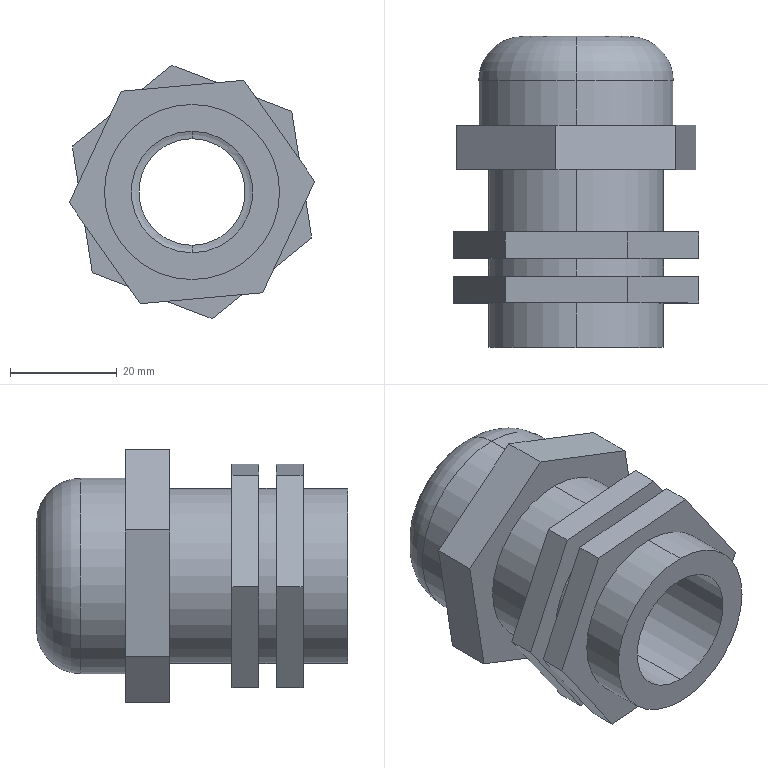Part | SolidWorks | features ICE 5, Extrusion 1, Fillet 1, Scale 1, Shell 1 | 1 solid | 44 faces | box 46.006 x 58.333 x 47.523 mm | volume 36742 mm3 | plane 26 | cylinder 14 | torus 4 | commonest cylinder face diameters 32.833 x6 20 x2 22.833 x2 26.667 x2 36.667 x2
STEP:
#1=CARTESIAN_POINT('',(0.,26.887,-11.417));
#2=VERTEX_POINT('',#1);
#3=CARTESIAN_POINT('',(0.,26.887,11.417));
#4=VERTEX_POINT('',#3);
#5=CARTESIAN_POINT('',(0.,26.887,0.));
#6=DIRECTION('',(0.,1.,0.));
#7=DIRECTION('',(0.,0.,1.));
#8=AXIS2_PLACEMENT_3D('',#5,#6,#7);
#9=CIRCLE('',#8,11.417);
#10=EDGE_CURVE('',#2,#4,#9,.T.);
#11=ORIENTED_EDGE('',*,*,#10,.T.);
#12=CARTESIAN_POINT('',(0.,-11.447,11.417));
#13=VERTEX_POINT('',#12);
#14=CARTESIAN_POINT('',(0.,21.887,11.417));
#15=DIRECTION('',(0.,-1.,0.));
#16=VECTOR('',#15,1000.);
#17=LINE('',#14,#16);
#18=EDGE_CURVE('',#4,#13,#17,.T.);
#19=ORIENTED_EDGE('',*,*,#18,.T.);
#20=CARTESIAN_POINT('',(0.,-11.447,-11.417));
#21=VERTEX_POINT('',#20);
#22=CARTESIAN_POINT('',(0.,-11.447,0.));
#23=DIRECTION('',(0.,1.,0.));
#24=DIRECTION('',(0.,0.,1.));
#25=AXIS2_PLACEMENT_3D('',#22,#23,#24);
#26=CIRCLE('',#25,11.417);
#27=EDGE_CURVE('',#21,#13,#26,.T.);
#28=ORIENTED_EDGE('',*,*,#27,.F.);
#29=CARTESIAN_POINT('',(0.,21.887,-11.417));
#30=DIRECTION('',(0.,-1.,0.));
#31=VECTOR('',#30,1000.);
#32=LINE('',#29,#31);
#33=EDGE_CURVE('',#2,#21,#32,.T.);
#34=ORIENTED_EDGE('',*,*,#33,.F.);
#35=EDGE_LOOP('',(#11,#19,#28,#34));
#36=FACE_OUTER_BOUND('',#35,.T.);
#37=CARTESIAN_POINT('',(0.,21.887,0.));
#38=DIRECTION('',(0.,-1.,0.));
#39=DIRECTION('',(0.,0.,-1.));
#40=AXIS2_PLACEMENT_3D('',#37,#38,#39);
#41=CYLINDRICAL_SURFACE('',#40,11.417);
#42=ADVANCED_FACE('',(#36),#41,.F.);
#43=CARTESIAN_POINT('',(0.,-3.113,-16.417));
#44=VERTEX_POINT('',#43);
#45=CARTESIAN_POINT('',(0.,-3.113,16.417));
#46=VERTEX_POINT('',#45);
#47=CARTESIAN_POINT('',(0.,-3.113,0.));
#48=DIRECTION('',(0.,-1.,0.));
#49=DIRECTION('',(0.,0.,-1.));
#50=AXIS2_PLACEMENT_3D('',#47,#48,#49);
#51=CIRCLE('',#50,16.417);
#52=EDGE_CURVE('',#44,#46,#51,.T.);
#53=ORIENTED_EDGE('',*,*,#52,.T.);
#54=CARTESIAN_POINT('',(0.,-11.447,16.417));
#55=VERTEX_POINT('',#54);
#56=CARTESIAN_POINT('',(0.,21.887,16.417));
#57=DIRECTION('',(0.,-1.,0.));
#58=VECTOR('',#57,1000.);
#59=LINE('',#56,#58);
#60=EDGE_CURVE('',#46,#55,#59,.T.);
#61=ORIENTED_EDGE('',*,*,#60,.T.);
#62=CARTESIAN_POINT('',(0.,-11.447,-16.417));
#63=VERTEX_POINT('',#62);
#64=CARTESIAN_POINT('',(0.,-11.447,0.));
#65=DIRECTION('',(0.,1.,0.));
#66=DIRECTION('',(0.,0.,1.));
#67=AXIS2_PLACEMENT_3D('',#64,#65,#66);
#68=CIRCLE('',#67,16.417);
#69=EDGE_CURVE('',#55,#63,#68,.T.);
#70=ORIENTED_EDGE('',*,*,#69,.T.);
#71=CARTESIAN_POINT('',(0.,21.887,-16.417));
#72=DIRECTION('',(0.,-1.,0.));
#73=VECTOR('',#72,1000.);
#74=LINE('',#71,#73);
#75=EDGE_CURVE('',#44,#63,#74,.T.);
#76=ORIENTED_EDGE('',*,*,#75,.F.);
#77=EDGE_LOOP('',(#53,#61,#70,#76));
#78=FACE_OUTER_BOUND('',#77,.T.);
#79=CARTESIAN_POINT('',(0.,21.887,0.));
#80=DIRECTION('',(0.,-1.,0.));
#81=DIRECTION('',(0.,0.,-1.));
#82=AXIS2_PLACEMENT_3D('',#79,#80,#81);
#83=CYLINDRICAL_SURFACE('',#82,16.417);
#84=ADVANCED_FACE('',(#78),#83,.T.);
#85=CARTESIAN_POINT('',(0.,38.553,13.333));
#86=VERTEX_POINT('',#85);
#87=CARTESIAN_POINT('',(0.,38.553,-13.333));
#88=VERTEX_POINT('',#87);
#89=CARTESIAN_POINT('',(0.,38.553,0.));
#90=DIRECTION('',(0.,-1.,0.));
#91=DIRECTION('',(0.,0.,-1.));
#92=AXIS2_PLACEMENT_3D('',#89,#90,#91);
#93=CIRCLE('',#92,13.333);
#94=EDGE_CURVE('',#86,#88,#93,.T.);
#95=ORIENTED_EDGE('',*,*,#94,.T.);
#96=CARTESIAN_POINT('',(0.,41.887,-10.));
#97=VERTEX_POINT('',#96);
#98=CARTESIAN_POINT('',(0.,38.553,-10.));
#99=DIRECTION('',(1.,0.,0.));
#100=DIRECTION('',(0.,0.,-1.));
#101=AXIS2_PLACEMENT_3D('',#98,#99,#100);
#102=CIRCLE('',#101,3.333);
#103=EDGE_CURVE('',#88,#97,#102,.T.);
#104=ORIENTED_EDGE('',*,*,#103,.T.);
#105=CARTESIAN_POINT('',(0.,41.887,10.));
#106=VERTEX_POINT('',#105);
#107=CARTESIAN_POINT('',(0.,41.887,0.));
#108=DIRECTION('',(0.,1.,0.));
#109=DIRECTION('',(0.,0.,-1.));
#110=AXIS2_PLACEMENT_3D('',#107,#108,#109);
#111=CIRCLE('',#110,10.);
#112=EDGE_CURVE('',#97,#106,#111,.T.);
#113=ORIENTED_EDGE('',*,*,#112,.T.);
#114=CARTESIAN_POINT('',(0.,38.553,10.));
#115=DIRECTION('',(-1.,0.,0.));
#116=DIRECTION('',(0.,0.,1.));
#117=AXIS2_PLACEMENT_3D('',#114,#115,#116);
#118=CIRCLE('',#117,3.333);
#119=EDGE_CURVE('',#86,#106,#118,.T.);
#120=ORIENTED_EDGE('',*,*,#119,.F.);
#121=EDGE_LOOP('',(#95,#104,#113,#120));
#122=FACE_OUTER_BOUND('',#121,.T.);
#123=CARTESIAN_POINT('',(0.,38.553,0.));
#124=DIRECTION('',(0.,1.,0.));
#125=DIRECTION('',(0.,0.,1.));
#126=AXIS2_PLACEMENT_3D('',#123,#124,#125);
#127=TOROIDAL_SURFACE('',#126,10.,3.333);
#128=ADVANCED_FACE('',(#122),#127,.F.);
#129=ORIENTED_EDGE('',*,*,#94,.F.);
#130=CARTESIAN_POINT('',(0.,26.887,13.333));
#131=VERTEX_POINT('',#130);
#132=CARTESIAN_POINT('',(0.,46.887,13.333));
#133=DIRECTION('',(0.,-1.,0.));
#134=VECTOR('',#133,1000.);
#135=LINE('',#132,#134);
#136=EDGE_CURVE('',#86,#131,#135,.T.);
#137=ORIENTED_EDGE('',*,*,#136,.T.);
#138=CARTESIAN_POINT('',(0.,26.887,-13.333));
#139=VERTEX_POINT('',#138);
#140=CARTESIAN_POINT('',(0.,26.887,0.));
#141=DIRECTION('',(0.,-1.,0.));
#142=DIRECTION('',(0.,0.,1.));
#143=AXIS2_PLACEMENT_3D('',#140,#141,#142);
#144=CIRCLE('',#143,13.333);
#145=EDGE_CURVE('',#131,#139,#144,.T.);
#146=ORIENTED_EDGE('',*,*,#145,.T.);
#147=CARTESIAN_POINT('',(0.,46.887,-13.333));
#148=DIRECTION('',(0.,-1.,0.));
#149=VECTOR('',#148,1000.);
#150=LINE('',#147,#149);
#151=EDGE_CURVE('',#88,#139,#150,.T.);
#152=ORIENTED_EDGE('',*,*,#151,.F.);
#153=EDGE_LOOP('',(#129,#137,#146,#152));
#154=FACE_OUTER_BOUND('',#153,.T.);
#155=CARTESIAN_POINT('',(0.,46.887,0.));
#156=DIRECTION('',(0.,-1.,0.));
#157=DIRECTION('',(0.,0.,-1.));
#158=AXIS2_PLACEMENT_3D('',#155,#156,#157);
#159=CYLINDRICAL_SURFACE('',#158,13.333);
#160=ADVANCED_FACE('',(#154),#159,.F.);
#161=ORIENTED_EDGE('',*,*,#112,.F.);
#162=CARTESIAN_POINT('',(0.,46.887,-10.));
#163=VERTEX_POINT('',#162);
#164=CARTESIAN_POINT('',(0.,46.887,-10.));
#165=DIRECTION('',(0.,1.,0.));
#166=VECTOR('',#165,1000.);
#167=LINE('',#164,#166);
#168=EDGE_CURVE('',#97,#163,#167,.T.);
#169=ORIENTED_EDGE('',*,*,#168,.T.);
#170=CARTESIAN_POINT('',(0.,46.887,10.));
#171=VERTEX_POINT('',#170);
#172=CARTESIAN_POINT('',(0.,46.887,0.));
#173=DIRECTION('',(0.,1.,0.));
#174=DIRECTION('',(0.,0.,1.));
#175=AXIS2_PLACEMENT_3D('',#172,#173,#174);
#176=CIRCLE('',#175,10.);
#177=EDGE_CURVE('',#163,#171,#176,.T.);
#178=ORIENTED_EDGE('',*,*,#177,.T.);
#179=CARTESIAN_POINT('',(0.,46.887,10.));
#180=DIRECTION('',(0.,1.,0.));
#181=VECTOR('',#180,1000.);
#182=LINE('',#179,#181);
#183=EDGE_CURVE('',#106,#171,#182,.T.);
#184=ORIENTED_EDGE('',*,*,#183,.F.);
#185=EDGE_LOOP('',(#161,#169,#178,#184));
#186=FACE_OUTER_BOUND('',#185,.T.);
#187=CARTESIAN_POINT('',(0.,46.887,0.));
#188=DIRECTION('',(0.,1.,0.));
#189=DIRECTION('',(0.,0.,1.));
#190=AXIS2_PLACEMENT_3D('',#187,#188,#189);
#191=CYLINDRICAL_SURFACE('',#190,10.);
#192=ADVANCED_FACE('',(#186),#191,.F.);
#193=CARTESIAN_POINT('',(0.,38.553,-18.333));
#194=VERTEX_POINT('',#193);
#195=CARTESIAN_POINT('',(0.,38.553,18.333));
#196=VERTEX_POINT('',#195);
#197=CARTESIAN_POINT('',(0.,38.553,0.));
#198=DIRECTION('',(0.,-1.,0.));
#199=DIRECTION('',(0.,0.,1.));
#200=AXIS2_PLACEMENT_3D('',#197,#198,#199);
#201=CIRCLE('',#200,18.333);
#202=EDGE_CURVE('',#194,#196,#201,.T.);
#203=ORIENTED_EDGE('',*,*,#202,.F.);
#204=CARTESIAN_POINT('',(0.,38.553,-10.));
#205=DIRECTION('',(1.,0.,0.));
#206=DIRECTION('',(0.,0.,-1.));
#207=AXIS2_PLACEMENT_3D('',#204,#205,#206);
#208=CIRCLE('',#207,8.333);
#209=EDGE_CURVE('',#194,#163,#208,.T.);
#210=ORIENTED_EDGE('',*,*,#209,.T.);
#211=CARTESIAN_POINT('',(0.,46.887,0.));
#212=DIRECTION('',(0.,1.,0.));
#213=DIRECTION('',(0.,0.,1.));
#214=AXIS2_PLACEMENT_3D('',#211,#212,#213);
#215=CIRCLE('',#214,10.);
#216=EDGE_CURVE('',#171,#163,#215,.T.);
#217=ORIENTED_EDGE('',*,*,#216,.F.);
#218=CARTESIAN_POINT('',(0.,38.553,10.));
#219=DIRECTION('',(-1.,0.,0.));
#220=DIRECTION('',(0.,0.,1.));
#221=AXIS2_PLACEMENT_3D('',#218,#219,#220);
#222=CIRCLE('',#221,8.333);
#223=EDGE_CURVE('',#196,#171,#222,.T.);
#224=ORIENTED_EDGE('',*,*,#223,.F.);
#225=EDGE_LOOP('',(#203,#210,#217,#224));
#226=FACE_OUTER_BOUND('',#225,.T.);
#227=CARTESIAN_POINT('',(0.,38.553,0.));
#228=DIRECTION('',(0.,1.,0.));
#229=DIRECTION('',(0.,0.,1.));
#230=AXIS2_PLACEMENT_3D('',#227,#228,#229);
#231=TOROIDAL_SURFACE('',#230,10.,8.333);
#232=ADVANCED_FACE('',(#226),#231,.T.);
#233=ORIENTED_EDGE('',*,*,#202,.T.);
#234=CARTESIAN_POINT('',(0.,30.22,18.333));
#235=VERTEX_POINT('',#234);
#236=CARTESIAN_POINT('',(0.,46.887,18.333));
#237=DIRECTION('',(0.,-1.,0.));
#238=VECTOR('',#237,1000.);
#239=LINE('',#236,#238);
#240=EDGE_CURVE('',#196,#235,#239,.T.);
#241=ORIENTED_EDGE('',*,*,#240,.T.);
#242=CARTESIAN_POINT('',(0.,30.22,-18.333));
#243=VERTEX_POINT('',#242);
#244=CARTESIAN_POINT('',(0.,30.22,0.));
#245=DIRECTION('',(0.,1.,0.));
#246=DIRECTION('',(0.,0.,1.));
#247=AXIS2_PLACEMENT_3D('',#244,#245,#246);
#248=CIRCLE('',#247,18.333);
#249=EDGE_CURVE('',#235,#243,#248,.T.);
#250=ORIENTED_EDGE('',*,*,#249,.T.);
#251=CARTESIAN_POINT('',(0.,46.887,-18.333));
#252=DIRECTION('',(0.,-1.,0.));
#253=VECTOR('',#252,1000.);
#254=LINE('',#251,#253);
#255=EDGE_CURVE('',#194,#243,#254,.T.);
#256=ORIENTED_EDGE('',*,*,#255,.F.);
#257=EDGE_LOOP('',(#233,#241,#250,#256));
#258=FACE_OUTER_BOUND('',#257,.T.);
#259=CARTESIAN_POINT('',(0.,46.887,0.));
#260=DIRECTION('',(0.,-1.,0.));
#261=DIRECTION('',(0.,0.,-1.));
#262=AXIS2_PLACEMENT_3D('',#259,#260,#261);
#263=CYLINDRICAL_SURFACE('',#262,18.333);
#264=ADVANCED_FACE('',(#258),#263,.T.);
#265=CARTESIAN_POINT('',(0.,21.887,16.417));
#266=VERTEX_POINT('',#265);
#267=CARTESIAN_POINT('',(0.,21.887,-16.417));
#268=VERTEX_POINT('',#267);
#269=CARTESIAN_POINT('',(0.,21.887,0.));
#270=DIRECTION('',(0.,1.,0.));
#271=DIRECTION('',(0.,0.,1.));
#272=AXIS2_PLACEMENT_3D('',#269,#270,#271);
#273=CIRCLE('',#272,16.417);
#274=EDGE_CURVE('',#266,#268,#273,.T.);
#275=ORIENTED_EDGE('',*,*,#274,.F.);
#276=CARTESIAN_POINT('',(0.,10.22,16.417));
#277=VERTEX_POINT('',#276);
#278=CARTESIAN_POINT('',(0.,21.887,16.417));
#279=DIRECTION('',(0.,-1.,0.));
#280=VECTOR('',#279,1000.);
#281=LINE('',#278,#280);
#282=EDGE_CURVE('',#266,#277,#281,.T.);
#283=ORIENTED_EDGE('',*,*,#282,.T.);
#284=CARTESIAN_POINT('',(0.,10.22,-16.417));
#285=VERTEX_POINT('',#284);
#286=CARTESIAN_POINT('',(0.,10.22,0.));
#287=DIRECTION('',(0.,-1.,0.));
#288=DIRECTION('',(0.,0.,-1.));
#289=AXIS2_PLACEMENT_3D('',#286,#287,#288);
#290=CIRCLE('',#289,16.417);
#291=EDGE_CURVE('',#285,#277,#290,.T.);
#292=ORIENTED_EDGE('',*,*,#291,.F.);
#293=CARTESIAN_POINT('',(0.,21.887,-16.417));
#294=DIRECTION('',(0.,-1.,0.));
#295=VECTOR('',#294,1000.);
#296=LINE('',#293,#295);
#297=EDGE_CURVE('',#268,#285,#296,.T.);
#298=ORIENTED_EDGE('',*,*,#297,.F.);
#299=EDGE_LOOP('',(#275,#283,#292,#298));
#300=FACE_OUTER_BOUND('',#299,.T.);
#301=CARTESIAN_POINT('',(0.,21.887,0.));
#302=DIRECTION('',(0.,-1.,0.));
#303=DIRECTION('',(0.,0.,-1.));
#304=AXIS2_PLACEMENT_3D('',#301,#302,#303);
#305=CYLINDRICAL_SURFACE('',#304,16.417);
#306=ADVANCED_FACE('',(#300),#305,.T.);
#307=CARTESIAN_POINT('',(0.,5.22,-16.417));
#308=VERTEX_POINT('',#307);
#309=CARTESIAN_POINT('',(0.,5.22,16.417));
#310=VERTEX_POINT('',#309);
#311=CARTESIAN_POINT('',(0.,5.22,0.));
#312=DIRECTION('',(0.,-1.,0.));
#313=DIRECTION('',(0.,0.,-1.));
#314=AXIS2_PLACEMENT_3D('',#311,#312,#313);
#315=CIRCLE('',#314,16.417);
#316=EDGE_CURVE('',#308,#310,#315,.T.);
#317=ORIENTED_EDGE('',*,*,#316,.T.);
#318=CARTESIAN_POINT('',(0.,1.887,16.417));
#319=VERTEX_POINT('',#318);
#320=CARTESIAN_POINT('',(0.,21.887,16.417));
#321=DIRECTION('',(0.,-1.,0.));
#322=VECTOR('',#321,1000.);
#323=LINE('',#320,#322);
#324=EDGE_CURVE('',#310,#319,#323,.T.);
#325=ORIENTED_EDGE('',*,*,#324,.T.);
#326=CARTESIAN_POINT('',(0.,1.887,-16.417));
#327=VERTEX_POINT('',#326);
#328=CARTESIAN_POINT('',(0.,1.887,0.));
#329=DIRECTION('',(0.,-1.,0.));
#330=DIRECTION('',(0.,0.,-1.));
#331=AXIS2_PLACEMENT_3D('',#328,#329,#330);
#332=CIRCLE('',#331,16.417);
#333=EDGE_CURVE('',#327,#319,#332,.T.);
#334=ORIENTED_EDGE('',*,*,#333,.F.);
#335=CARTESIAN_POINT('',(0.,21.887,-16.417));
#336=DIRECTION('',(0.,-1.,0.));
#337=VECTOR('',#336,1000.);
#338=LINE('',#335,#337);
#339=EDGE_CURVE('',#308,#327,#338,.T.);
#340=ORIENTED_EDGE('',*,*,#339,.F.);
#341=EDGE_LOOP('',(#317,#325,#334,#340));
#342=FACE_OUTER_BOUND('',#341,.T.);
#343=CARTESIAN_POINT('',(0.,21.887,0.));
#344=DIRECTION('',(0.,-1.,0.));
#345=DIRECTION('',(0.,0.,-1.));
#346=AXIS2_PLACEMENT_3D('',#343,#344,#345);
#347=CYLINDRICAL_SURFACE('',#346,16.417);
#348=ADVANCED_FACE('',(#342),#347,.T.);
#349=ORIENTED_EDGE('',*,*,#324,.F.);
#350=CARTESIAN_POINT('',(0.,5.22,0.));
#351=DIRECTION('',(0.,-1.,0.));
#352=DIRECTION('',(0.,0.,-1.));
#353=AXIS2_PLACEMENT_3D('',#350,#351,#352);
#354=CIRCLE('',#353,16.417);
#355=EDGE_CURVE('',#310,#308,#354,.T.);
#356=ORIENTED_EDGE('',*,*,#355,.T.);
#357=ORIENTED_EDGE('',*,*,#339,.T.);
#358=CARTESIAN_POINT('',(0.,1.887,0.));
#359=DIRECTION('',(0.,-1.,0.));
#360=DIRECTION('',(0.,0.,-1.));
#361=AXIS2_PLACEMENT_3D('',#358,#359,#360);
#362=CIRCLE('',#361,16.417);
#363=EDGE_CURVE('',#319,#327,#362,.T.);
#364=ORIENTED_EDGE('',*,*,#363,.F.);
#365=EDGE_LOOP('',(#349,#356,#357,#364));
#366=FACE_OUTER_BOUND('',#365,.T.);
#367=CARTESIAN_POINT('',(0.,21.887,0.));
#368=DIRECTION('',(0.,-1.,0.));
#369=DIRECTION('',(0.,0.,-1.));
#370=AXIS2_PLACEMENT_3D('',#367,#368,#369);
#371=CYLINDRICAL_SURFACE('',#370,16.417);
#372=ADVANCED_FACE('',(#366),#371,.T.);
#373=ORIENTED_EDGE('',*,*,#282,.F.);
#374=CARTESIAN_POINT('',(0.,21.887,0.));
#375=DIRECTION('',(0.,1.,0.));
#376=DIRECTION('',(0.,0.,1.));
#377=AXIS2_PLACEMENT_3D('',#374,#375,#376);
#378=CIRCLE('',#377,16.417);
#379=EDGE_CURVE('',#268,#266,#378,.T.);
#380=ORIENTED_EDGE('',*,*,#379,.F.);
#381=ORIENTED_EDGE('',*,*,#297,.T.);
#382=CARTESIAN_POINT('',(0.,10.22,0.));
#383=DIRECTION('',(0.,-1.,0.));
#384=DIRECTION('',(0.,0.,-1.));
#385=AXIS2_PLACEMENT_3D('',#382,#383,#384);
#386=CIRCLE('',#385,16.417);
#387=EDGE_CURVE('',#277,#285,#386,.T.);
#388=ORIENTED_EDGE('',*,*,#387,.F.);
#389=EDGE_LOOP('',(#373,#380,#381,#388));
#390=FACE_OUTER_BOUND('',#389,.T.);
#391=CARTESIAN_POINT('',(0.,21.887,0.));
#392=DIRECTION('',(0.,-1.,0.));
#393=DIRECTION('',(0.,0.,-1.));
#394=AXIS2_PLACEMENT_3D('',#391,#392,#393);
#395=CYLINDRICAL_SURFACE('',#394,16.417);
#396=ADVANCED_FACE('',(#390),#395,.T.);
#397=CARTESIAN_POINT('',(22.455,21.887,-8.629));
#398=VERTEX_POINT('',#397);
#399=CARTESIAN_POINT('',(3.754,21.887,-23.761));
#400=VERTEX_POINT('',#399);
#401=CARTESIAN_POINT('',(22.455,21.887,-8.629));
#402=DIRECTION('',(-0.7774,0.,-0.629));
#403=VECTOR('',#402,1000.);
#404=LINE('',#401,#403);
#405=EDGE_CURVE('',#398,#400,#404,.T.);
#406=ORIENTED_EDGE('',*,*,#405,.T.);
#407=CARTESIAN_POINT('',(3.754,30.22,-23.761));
#408=VERTEX_POINT('',#407);
#409=CARTESIAN_POINT('',(3.754,30.22,-23.761));
#410=DIRECTION('',(0.,-1.,0.));
#411=VECTOR('',#410,1000.);
#412=LINE('',#409,#411);
#413=EDGE_CURVE('',#408,#400,#412,.T.);
#414=ORIENTED_EDGE('',*,*,#413,.F.);
#415=CARTESIAN_POINT('',(22.455,30.22,-8.629));
#416=VERTEX_POINT('',#415);
#417=CARTESIAN_POINT('',(22.455,30.22,-8.629));
#418=DIRECTION('',(-0.7774,0.,-0.629));
#419=VECTOR('',#418,1000.);
#420=LINE('',#417,#419);
#421=EDGE_CURVE('',#416,#408,#420,.T.);
#422=ORIENTED_EDGE('',*,*,#421,.F.);
#423=CARTESIAN_POINT('',(22.455,30.22,-8.629));
#424=DIRECTION('',(0.,-1.,0.));
#425=VECTOR('',#424,1000.);
#426=LINE('',#423,#425);
#427=EDGE_CURVE('',#416,#398,#426,.T.);
#428=ORIENTED_EDGE('',*,*,#427,.T.);
#429=EDGE_LOOP('',(#406,#414,#422,#428));
#430=FACE_OUTER_BOUND('',#429,.T.);
#431=CARTESIAN_POINT('',(22.455,30.22,-8.629));
#432=DIRECTION('',(-0.629,0.,0.7774));
#433=DIRECTION('',(0.7774,0.,0.629));
#434=AXIS2_PLACEMENT_3D('',#431,#432,#433);
#435=PLANE('',#434);
#436=ADVANCED_FACE('',(#430),#435,.F.);
#437=CARTESIAN_POINT('',(-18.701,21.887,-15.132));
#438=VERTEX_POINT('',#437);
#439=CARTESIAN_POINT('',(3.754,21.887,-23.761));
#440=DIRECTION('',(-0.9334,0.,0.3587));
#441=VECTOR('',#440,1000.);
#442=LINE('',#439,#441);
#443=EDGE_CURVE('',#400,#438,#442,.T.);
#444=ORIENTED_EDGE('',*,*,#443,.T.);
#445=CARTESIAN_POINT('',(-18.701,30.22,-15.132));
#446=VERTEX_POINT('',#445);
#447=CARTESIAN_POINT('',(-18.701,30.22,-15.132));
#448=DIRECTION('',(0.,-1.,0.));
#449=VECTOR('',#448,1000.);
#450=LINE('',#447,#449);
#451=EDGE_CURVE('',#446,#438,#450,.T.);
#452=ORIENTED_EDGE('',*,*,#451,.F.);
#453=CARTESIAN_POINT('',(3.754,30.22,-23.761));
#454=DIRECTION('',(-0.9334,0.,0.3587));
#455=VECTOR('',#454,1000.);
#456=LINE('',#453,#455);
#457=EDGE_CURVE('',#408,#446,#456,.T.);
#458=ORIENTED_EDGE('',*,*,#457,.F.);
#459=ORIENTED_EDGE('',*,*,#413,.T.);
#460=EDGE_LOOP('',(#444,#452,#458,#459));
#461=FACE_OUTER_BOUND('',#460,.T.);
#462=CARTESIAN_POINT('',(3.754,30.22,-23.761));
#463=DIRECTION('',(0.3587,0.,0.9334));
#464=DIRECTION('',(0.9334,0.,-0.3587));
#465=AXIS2_PLACEMENT_3D('',#462,#463,#464);
#466=PLANE('',#465);
#467=ADVANCED_FACE('',(#461),#466,.F.);
#468=CARTESIAN_POINT('',(-22.455,21.887,8.629));
#469=VERTEX_POINT('',#468);
#470=CARTESIAN_POINT('',(-18.701,21.887,-15.132));
#471=DIRECTION('',(-0.1561,0.,0.9877));
#472=VECTOR('',#471,1000.);
#473=LINE('',#470,#472);
#474=EDGE_CURVE('',#438,#469,#473,.T.);
#475=ORIENTED_EDGE('',*,*,#474,.T.);
#476=CARTESIAN_POINT('',(-22.455,30.22,8.629));
#477=VERTEX_POINT('',#476);
#478=CARTESIAN_POINT('',(-22.455,30.22,8.629));
#479=DIRECTION('',(0.,-1.,0.));
#480=VECTOR('',#479,1000.);
#481=LINE('',#478,#480);
#482=EDGE_CURVE('',#477,#469,#481,.T.);
#483=ORIENTED_EDGE('',*,*,#482,.F.);
#484=CARTESIAN_POINT('',(-18.701,30.22,-15.132));
#485=DIRECTION('',(-0.1561,0.,0.9877));
#486=VECTOR('',#485,1000.);
#487=LINE('',#484,#486);
#488=EDGE_CURVE('',#446,#477,#487,.T.);
#489=ORIENTED_EDGE('',*,*,#488,.F.);
#490=ORIENTED_EDGE('',*,*,#451,.T.);
#491=EDGE_LOOP('',(#475,#483,#489,#490));
#492=FACE_OUTER_BOUND('',#491,.T.);
#493=CARTESIAN_POINT('',(-18.701,30.22,-15.132));
#494=DIRECTION('',(0.9877,0.,0.1561));
#495=DIRECTION('',(0.1561,0.,-0.9877));
#496=AXIS2_PLACEMENT_3D('',#493,#494,#495);
#497=PLANE('',#496);
#498=ADVANCED_FACE('',(#492),#497,.F.);
#499=CARTESIAN_POINT('',(-3.754,21.887,23.761));
#500=VERTEX_POINT('',#499);
#501=CARTESIAN_POINT('',(-22.455,21.887,8.629));
#502=DIRECTION('',(0.7774,0.,0.629));
#503=VECTOR('',#502,1000.);
#504=LINE('',#501,#503);
#505=EDGE_CURVE('',#469,#500,#504,.T.);
#506=ORIENTED_EDGE('',*,*,#505,.T.);
#507=CARTESIAN_POINT('',(-3.754,30.22,23.761));
#508=VERTEX_POINT('',#507);
#509=CARTESIAN_POINT('',(-3.754,30.22,23.761));
#510=DIRECTION('',(0.,-1.,0.));
#511=VECTOR('',#510,1000.);
#512=LINE('',#509,#511);
#513=EDGE_CURVE('',#508,#500,#512,.T.);
#514=ORIENTED_EDGE('',*,*,#513,.F.);
#515=CARTESIAN_POINT('',(-22.455,30.22,8.629));
#516=DIRECTION('',(0.7774,0.,0.629));
#517=VECTOR('',#516,1000.);
#518=LINE('',#515,#517);
#519=EDGE_CURVE('',#477,#508,#518,.T.);
#520=ORIENTED_EDGE('',*,*,#519,.F.);
#521=ORIENTED_EDGE('',*,*,#482,.T.);
#522=EDGE_LOOP('',(#506,#514,#520,#521));
#523=FACE_OUTER_BOUND('',#522,.T.);
#524=CARTESIAN_POINT('',(-22.455,30.22,8.629));
#525=DIRECTION('',(0.629,0.,-0.7774));
#526=DIRECTION('',(-0.7774,0.,-0.629));
#527=AXIS2_PLACEMENT_3D('',#524,#525,#526);
#528=PLANE('',#527);
#529=ADVANCED_FACE('',(#523),#528,.F.);
#530=CARTESIAN_POINT('',(18.701,21.887,15.132));
#531=VERTEX_POINT('',#530);
#532=CARTESIAN_POINT('',(-3.754,21.887,23.761));
#533=DIRECTION('',(0.9334,0.,-0.3587));
#534=VECTOR('',#533,1000.);
#535=LINE('',#532,#534);
#536=EDGE_CURVE('',#500,#531,#535,.T.);
#537=ORIENTED_EDGE('',*,*,#536,.T.);
#538=CARTESIAN_POINT('',(18.701,30.22,15.132));
#539=VERTEX_POINT('',#538);
#540=CARTESIAN_POINT('',(18.701,30.22,15.132));
#541=DIRECTION('',(0.,-1.,0.));
#542=VECTOR('',#541,1000.);
#543=LINE('',#540,#542);
#544=EDGE_CURVE('',#539,#531,#543,.T.);
#545=ORIENTED_EDGE('',*,*,#544,.F.);
#546=CARTESIAN_POINT('',(-3.754,30.22,23.761));
#547=DIRECTION('',(0.9334,0.,-0.3587));
#548=VECTOR('',#547,1000.);
#549=LINE('',#546,#548);
#550=EDGE_CURVE('',#508,#539,#549,.T.);
#551=ORIENTED_EDGE('',*,*,#550,.F.);
#552=ORIENTED_EDGE('',*,*,#513,.T.);
#553=EDGE_LOOP('',(#537,#545,#551,#552));
#554=FACE_OUTER_BOUND('',#553,.T.);
#555=CARTESIAN_POINT('',(-3.754,30.22,23.761));
#556=DIRECTION('',(-0.3587,0.,-0.9334));
#557=DIRECTION('',(-0.9334,0.,0.3587));
#558=AXIS2_PLACEMENT_3D('',#555,#556,#557);
#559=PLANE('',#558);
#560=ADVANCED_FACE('',(#554),#559,.F.);
#561=CARTESIAN_POINT('',(18.701,21.887,15.132));
#562=DIRECTION('',(0.1561,0.,-0.9877));
#563=VECTOR('',#562,1000.);
#564=LINE('',#561,#563);
#565=EDGE_CURVE('',#531,#398,#564,.T.);
#566=ORIENTED_EDGE('',*,*,#565,.T.);
#567=ORIENTED_EDGE('',*,*,#427,.F.);
#568=CARTESIAN_POINT('',(18.701,30.22,15.132));
#569=DIRECTION('',(0.1561,0.,-0.9877));
#570=VECTOR('',#569,1000.);
#571=LINE('',#568,#570);
#572=EDGE_CURVE('',#539,#416,#571,.T.);
#573=ORIENTED_EDGE('',*,*,#572,.F.);
#574=ORIENTED_EDGE('',*,*,#544,.T.);
#575=EDGE_LOOP('',(#566,#567,#573,#574));
#576=FACE_OUTER_BOUND('',#575,.T.);
#577=CARTESIAN_POINT('',(18.701,30.22,15.132));
#578=DIRECTION('',(-0.9877,0.,-0.1561));
#579=DIRECTION('',(-0.1561,0.,0.9877));
#580=AXIS2_PLACEMENT_3D('',#577,#578,#579);
#581=PLANE('',#580);
#582=ADVANCED_FACE('',(#576),#581,.F.);
#583=CARTESIAN_POINT('',(0.,30.22,0.));
#584=DIRECTION('',(0.,1.,0.));
#585=DIRECTION('',(0.,0.,1.));
#586=AXIS2_PLACEMENT_3D('',#583,#584,#585);
#587=CIRCLE('',#586,18.333);
#588=EDGE_CURVE('',#243,#235,#587,.T.);
#589=ORIENTED_EDGE('',*,*,#588,.F.);
#590=ORIENTED_EDGE('',*,*,#249,.F.);
#591=EDGE_LOOP('',(#589,#590));
#592=FACE_BOUND('',#591,.T.);
#593=ORIENTED_EDGE('',*,*,#421,.T.);
#594=ORIENTED_EDGE('',*,*,#457,.T.);
#595=ORIENTED_EDGE('',*,*,#488,.T.);
#596=ORIENTED_EDGE('',*,*,#519,.T.);
#597=ORIENTED_EDGE('',*,*,#550,.T.);
#598=ORIENTED_EDGE('',*,*,#572,.T.);
#599=EDGE_LOOP('',(#593,#594,#595,#596,#597,#598));
#600=FACE_OUTER_BOUND('',#599,.T.);
#601=CARTESIAN_POINT('',(0.,30.22,0.));
#602=DIRECTION('',(0.,1.,0.));
#603=DIRECTION('',(0.,0.,1.));
#604=AXIS2_PLACEMENT_3D('',#601,#602,#603);
#605=PLANE('',#604);
#606=ADVANCED_FACE('',(#592,#600),#605,.T.);
#607=ORIENTED_EDGE('',*,*,#379,.T.);
#608=ORIENTED_EDGE('',*,*,#274,.T.);
#609=EDGE_LOOP('',(#607,#608));
#610=FACE_BOUND('',#609,.T.);
#611=ORIENTED_EDGE('',*,*,#405,.F.);
#612=ORIENTED_EDGE('',*,*,#565,.F.);
#613=ORIENTED_EDGE('',*,*,#536,.F.);
#614=ORIENTED_EDGE('',*,*,#505,.F.);
#615=ORIENTED_EDGE('',*,*,#474,.F.);
#616=ORIENTED_EDGE('',*,*,#443,.F.);
#617=EDGE_LOOP('',(#611,#612,#613,#614,#615,#616));
#618=FACE_OUTER_BOUND('',#617,.T.);
#619=CARTESIAN_POINT('',(0.,21.887,0.));
#620=DIRECTION('',(0.,1.,0.));
#621=DIRECTION('',(0.,0.,1.));
#622=AXIS2_PLACEMENT_3D('',#619,#620,#621);
#623=PLANE('',#622);
#624=ADVANCED_FACE('',(#610,#618),#623,.F.);
#625=ORIENTED_EDGE('',*,*,#240,.F.);
#626=CARTESIAN_POINT('',(0.,38.553,0.));
#627=DIRECTION('',(0.,-1.,0.));
#628=DIRECTION('',(0.,0.,1.));
#629=AXIS2_PLACEMENT_3D('',#626,#627,#628);
#630=CIRCLE('',#629,18.333);
#631=EDGE_CURVE('',#196,#194,#630,.T.);
#632=ORIENTED_EDGE('',*,*,#631,.T.);
#633=ORIENTED_EDGE('',*,*,#255,.T.);
#634=ORIENTED_EDGE('',*,*,#588,.T.);
#635=EDGE_LOOP('',(#625,#632,#633,#634));
#636=FACE_OUTER_BOUND('',#635,.T.);
#637=CARTESIAN_POINT('',(0.,46.887,0.));
#638=DIRECTION('',(0.,-1.,0.));
#639=DIRECTION('',(0.,0.,-1.));
#640=AXIS2_PLACEMENT_3D('',#637,#638,#639);
#641=CYLINDRICAL_SURFACE('',#640,18.333);
#642=ADVANCED_FACE('',(#636),#641,.T.);
#643=ORIENTED_EDGE('',*,*,#209,.F.);
#644=ORIENTED_EDGE('',*,*,#631,.F.);
#645=ORIENTED_EDGE('',*,*,#223,.T.);
#646=ORIENTED_EDGE('',*,*,#177,.F.);
#647=EDGE_LOOP('',(#643,#644,#645,#646));
#648=FACE_OUTER_BOUND('',#647,.T.);
#649=CARTESIAN_POINT('',(0.,38.553,0.));
#650=DIRECTION('',(0.,1.,0.));
#651=DIRECTION('',(0.,0.,1.));
#652=AXIS2_PLACEMENT_3D('',#649,#650,#651);
#653=TOROIDAL_SURFACE('',#652,10.,8.333);
#654=ADVANCED_FACE('',(#648),#653,.T.);
#655=ORIENTED_EDGE('',*,*,#10,.F.);
#656=CARTESIAN_POINT('',(0.,26.887,0.));
#657=DIRECTION('',(0.,1.,0.));
#658=DIRECTION('',(0.,0.,1.));
#659=AXIS2_PLACEMENT_3D('',#656,#657,#658);
#660=CIRCLE('',#659,11.417);
#661=EDGE_CURVE('',#4,#2,#660,.T.);
#662=ORIENTED_EDGE('',*,*,#661,.F.);
#663=EDGE_LOOP('',(#655,#662));
#664=FACE_BOUND('',#663,.T.);
#665=CARTESIAN_POINT('',(0.,26.887,0.));
#666=DIRECTION('',(0.,-1.,0.));
#667=DIRECTION('',(0.,0.,1.));
#668=AXIS2_PLACEMENT_3D('',#665,#666,#667);
#669=CIRCLE('',#668,13.333);
#670=EDGE_CURVE('',#139,#131,#669,.T.);
#671=ORIENTED_EDGE('',*,*,#670,.F.);
#672=ORIENTED_EDGE('',*,*,#145,.F.);
#673=EDGE_LOOP('',(#671,#672));
#674=FACE_OUTER_BOUND('',#673,.T.);
#675=CARTESIAN_POINT('',(0.,26.887,0.));
#676=DIRECTION('',(0.,1.,0.));
#677=DIRECTION('',(0.,0.,1.));
#678=AXIS2_PLACEMENT_3D('',#675,#676,#677);
#679=PLANE('',#678);
#680=ADVANCED_FACE('',(#664,#674),#679,.T.);
#681=ORIENTED_EDGE('',*,*,#168,.F.);
#682=CARTESIAN_POINT('',(0.,41.887,0.));
#683=DIRECTION('',(0.,1.,0.));
#684=DIRECTION('',(0.,0.,-1.));
#685=AXIS2_PLACEMENT_3D('',#682,#683,#684);
#686=CIRCLE('',#685,10.);
#687=EDGE_CURVE('',#106,#97,#686,.T.);
#688=ORIENTED_EDGE('',*,*,#687,.F.);
#689=ORIENTED_EDGE('',*,*,#183,.T.);
#690=ORIENTED_EDGE('',*,*,#216,.T.);
#691=EDGE_LOOP('',(#681,#688,#689,#690));
#692=FACE_OUTER_BOUND('',#691,.T.);
#693=CARTESIAN_POINT('',(0.,46.887,0.));
#694=DIRECTION('',(0.,1.,0.));
#695=DIRECTION('',(0.,0.,1.));
#696=AXIS2_PLACEMENT_3D('',#693,#694,#695);
#697=CYLINDRICAL_SURFACE('',#696,10.);
#698=ADVANCED_FACE('',(#692),#697,.F.);
#699=ORIENTED_EDGE('',*,*,#136,.F.);
#700=CARTESIAN_POINT('',(0.,38.553,0.));
#701=DIRECTION('',(0.,-1.,0.));
#702=DIRECTION('',(0.,0.,-1.));
#703=AXIS2_PLACEMENT_3D('',#700,#701,#702);
#704=CIRCLE('',#703,13.333);
#705=EDGE_CURVE('',#88,#86,#704,.T.);
#706=ORIENTED_EDGE('',*,*,#705,.F.);
#707=ORIENTED_EDGE('',*,*,#151,.T.);
#708=ORIENTED_EDGE('',*,*,#670,.T.);
#709=EDGE_LOOP('',(#699,#706,#707,#708));
#710=FACE_OUTER_BOUND('',#709,.T.);
#711=CARTESIAN_POINT('',(0.,46.887,0.));
#712=DIRECTION('',(0.,-1.,0.));
#713=DIRECTION('',(0.,0.,-1.));
#714=AXIS2_PLACEMENT_3D('',#711,#712,#713);
#715=CYLINDRICAL_SURFACE('',#714,13.333);
#716=ADVANCED_FACE('',(#710),#715,.F.);
#717=ORIENTED_EDGE('',*,*,#103,.F.);
#718=ORIENTED_EDGE('',*,*,#705,.T.);
#719=ORIENTED_EDGE('',*,*,#119,.T.);
#720=ORIENTED_EDGE('',*,*,#687,.T.);
#721=EDGE_LOOP('',(#717,#718,#719,#720));
#722=FACE_OUTER_BOUND('',#721,.T.);
#723=CARTESIAN_POINT('',(0.,38.553,0.));
#724=DIRECTION('',(0.,1.,0.));
#725=DIRECTION('',(0.,0.,1.));
#726=AXIS2_PLACEMENT_3D('',#723,#724,#725);
#727=TOROIDAL_SURFACE('',#726,10.,3.333);
#728=ADVANCED_FACE('',(#722),#727,.F.);
#729=CARTESIAN_POINT('',(-23.003,5.22,-2.048));
#730=VERTEX_POINT('',#729);
#731=CARTESIAN_POINT('',(-9.728,5.22,-20.945));
#732=VERTEX_POINT('',#731);
#733=CARTESIAN_POINT('',(-23.003,5.22,-2.048));
#734=DIRECTION('',(0.5748,0.,-0.8183));
#735=VECTOR('',#734,1000.);
#736=LINE('',#733,#735);
#737=EDGE_CURVE('',#730,#732,#736,.T.);
#738=ORIENTED_EDGE('',*,*,#737,.F.);
#739=CARTESIAN_POINT('',(-23.003,10.22,-2.048));
#740=VERTEX_POINT('',#739);
#741=CARTESIAN_POINT('',(-23.003,10.22,-2.048));
#742=DIRECTION('',(0.,-1.,0.));
#743=VECTOR('',#742,1000.);
#744=LINE('',#741,#743);
#745=EDGE_CURVE('',#740,#730,#744,.T.);
#746=ORIENTED_EDGE('',*,*,#745,.F.);
#747=CARTESIAN_POINT('',(-9.728,10.22,-20.945));
#748=VERTEX_POINT('',#747);
#749=CARTESIAN_POINT('',(-23.003,10.22,-2.048));
#750=DIRECTION('',(0.5748,0.,-0.8183));
#751=VECTOR('',#750,1000.);
#752=LINE('',#749,#751);
#753=EDGE_CURVE('',#740,#748,#752,.T.);
#754=ORIENTED_EDGE('',*,*,#753,.T.);
#755=CARTESIAN_POINT('',(-9.728,10.22,-20.945));
#756=DIRECTION('',(0.,-1.,0.));
#757=VECTOR('',#756,1000.);
#758=LINE('',#755,#757);
#759=EDGE_CURVE('',#748,#732,#758,.T.);
#760=ORIENTED_EDGE('',*,*,#759,.T.);
#761=EDGE_LOOP('',(#738,#746,#754,#760));
#762=FACE_OUTER_BOUND('',#761,.T.);
#763=CARTESIAN_POINT('',(-23.003,10.22,-2.048));
#764=DIRECTION('',(-0.8183,0.,-0.5748));
#765=DIRECTION('',(-0.5748,0.,0.8183));
#766=AXIS2_PLACEMENT_3D('',#763,#764,#765);
#767=PLANE('',#766);
#768=ADVANCED_FACE('',(#762),#767,.T.);
#769=CARTESIAN_POINT('',(-13.275,5.22,18.897));
#770=VERTEX_POINT('',#769);
#771=CARTESIAN_POINT('',(-13.275,5.22,18.897));
#772=DIRECTION('',(-0.4212,0.,-0.907));
#773=VECTOR('',#772,1000.);
#774=LINE('',#771,#773);
#775=EDGE_CURVE('',#770,#730,#774,.T.);
#776=ORIENTED_EDGE('',*,*,#775,.F.);
#777=CARTESIAN_POINT('',(-13.275,10.22,18.897));
#778=VERTEX_POINT('',#777);
#779=CARTESIAN_POINT('',(-13.275,10.22,18.897));
#780=DIRECTION('',(0.,-1.,0.));
#781=VECTOR('',#780,1000.);
#782=LINE('',#779,#781);
#783=EDGE_CURVE('',#778,#770,#782,.T.);
#784=ORIENTED_EDGE('',*,*,#783,.F.);
#785=CARTESIAN_POINT('',(-13.275,10.22,18.897));
#786=DIRECTION('',(-0.4212,0.,-0.907));
#787=VECTOR('',#786,1000.);
#788=LINE('',#785,#787);
#789=EDGE_CURVE('',#778,#740,#788,.T.);
#790=ORIENTED_EDGE('',*,*,#789,.T.);
#791=ORIENTED_EDGE('',*,*,#745,.T.);
#792=EDGE_LOOP('',(#776,#784,#790,#791));
#793=FACE_OUTER_BOUND('',#792,.T.);
#794=CARTESIAN_POINT('',(-13.275,10.22,18.897));
#795=DIRECTION('',(-0.907,0.,0.4212));
#796=DIRECTION('',(0.4212,0.,0.907));
#797=AXIS2_PLACEMENT_3D('',#794,#795,#796);
#798=PLANE('',#797);
#799=ADVANCED_FACE('',(#793),#798,.T.);
#800=CARTESIAN_POINT('',(9.728,5.22,20.945));
#801=VERTEX_POINT('',#800);
#802=CARTESIAN_POINT('',(9.728,5.22,20.945));
#803=DIRECTION('',(-0.9961,0.,-0.08869));
#804=VECTOR('',#803,1000.);
#805=LINE('',#802,#804);
#806=EDGE_CURVE('',#801,#770,#805,.T.);
#807=ORIENTED_EDGE('',*,*,#806,.F.);
#808=CARTESIAN_POINT('',(9.728,10.22,20.945));
#809=VERTEX_POINT('',#808);
#810=CARTESIAN_POINT('',(9.728,10.22,20.945));
#811=DIRECTION('',(0.,-1.,0.));
#812=VECTOR('',#811,1000.);
#813=LINE('',#810,#812);
#814=EDGE_CURVE('',#809,#801,#813,.T.);
#815=ORIENTED_EDGE('',*,*,#814,.F.);
#816=CARTESIAN_POINT('',(9.728,10.22,20.945));
#817=DIRECTION('',(-0.9961,0.,-0.08869));
#818=VECTOR('',#817,1000.);
#819=LINE('',#816,#818);
#820=EDGE_CURVE('',#809,#778,#819,.T.);
#821=ORIENTED_EDGE('',*,*,#820,.T.);
#822=ORIENTED_EDGE('',*,*,#783,.T.);
#823=EDGE_LOOP('',(#807,#815,#821,#822));
#824=FACE_OUTER_BOUND('',#823,.T.);
#825=CARTESIAN_POINT('',(9.728,10.22,20.945));
#826=DIRECTION('',(-0.08869,0.,0.9961));
#827=DIRECTION('',(0.9961,0.,0.08869));
#828=AXIS2_PLACEMENT_3D('',#825,#826,#827);
#829=PLANE('',#828);
#830=ADVANCED_FACE('',(#824),#829,.T.);
#831=CARTESIAN_POINT('',(23.003,5.22,2.048));
#832=VERTEX_POINT('',#831);
#833=CARTESIAN_POINT('',(23.003,5.22,2.048));
#834=DIRECTION('',(-0.5748,0.,0.8183));
#835=VECTOR('',#834,1000.);
#836=LINE('',#833,#835);
#837=EDGE_CURVE('',#832,#801,#836,.T.);
#838=ORIENTED_EDGE('',*,*,#837,.F.);
#839=CARTESIAN_POINT('',(23.003,10.22,2.048));
#840=VERTEX_POINT('',#839);
#841=CARTESIAN_POINT('',(23.003,10.22,2.048));
#842=DIRECTION('',(0.,-1.,0.));
#843=VECTOR('',#842,1000.);
#844=LINE('',#841,#843);
#845=EDGE_CURVE('',#840,#832,#844,.T.);
#846=ORIENTED_EDGE('',*,*,#845,.F.);
#847=CARTESIAN_POINT('',(23.003,10.22,2.048));
#848=DIRECTION('',(-0.5748,0.,0.8183));
#849=VECTOR('',#848,1000.);
#850=LINE('',#847,#849);
#851=EDGE_CURVE('',#840,#809,#850,.T.);
#852=ORIENTED_EDGE('',*,*,#851,.T.);
#853=ORIENTED_EDGE('',*,*,#814,.T.);
#854=EDGE_LOOP('',(#838,#846,#852,#853));
#855=FACE_OUTER_BOUND('',#854,.T.);
#856=CARTESIAN_POINT('',(23.003,10.22,2.048));
#857=DIRECTION('',(0.8183,0.,0.5748));
#858=DIRECTION('',(0.5748,0.,-0.8183));
#859=AXIS2_PLACEMENT_3D('',#856,#857,#858);
#860=PLANE('',#859);
#861=ADVANCED_FACE('',(#855),#860,.T.);
#862=CARTESIAN_POINT('',(13.275,5.22,-18.897));
#863=VERTEX_POINT('',#862);
#864=CARTESIAN_POINT('',(13.275,5.22,-18.897));
#865=DIRECTION('',(0.4212,0.,0.907));
#866=VECTOR('',#865,1000.);
#867=LINE('',#864,#866);
#868=EDGE_CURVE('',#863,#832,#867,.T.);
#869=ORIENTED_EDGE('',*,*,#868,.F.);
#870=CARTESIAN_POINT('',(13.275,10.22,-18.897));
#871=VERTEX_POINT('',#870);
#872=CARTESIAN_POINT('',(13.275,10.22,-18.897));
#873=DIRECTION('',(0.,-1.,0.));
#874=VECTOR('',#873,1000.);
#875=LINE('',#872,#874);
#876=EDGE_CURVE('',#871,#863,#875,.T.);
#877=ORIENTED_EDGE('',*,*,#876,.F.);
#878=CARTESIAN_POINT('',(13.275,10.22,-18.897));
#879=DIRECTION('',(0.4212,0.,0.907));
#880=VECTOR('',#879,1000.);
#881=LINE('',#878,#880);
#882=EDGE_CURVE('',#871,#840,#881,.T.);
#883=ORIENTED_EDGE('',*,*,#882,.T.);
#884=ORIENTED_EDGE('',*,*,#845,.T.);
#885=EDGE_LOOP('',(#869,#877,#883,#884));
#886=FACE_OUTER_BOUND('',#885,.T.);
#887=CARTESIAN_POINT('',(13.275,10.22,-18.897));
#888=DIRECTION('',(0.907,0.,-0.4212));
#889=DIRECTION('',(-0.4212,0.,-0.907));
#890=AXIS2_PLACEMENT_3D('',#887,#888,#889);
#891=PLANE('',#890);
#892=ADVANCED_FACE('',(#886),#891,.T.);
#893=CARTESIAN_POINT('',(-9.728,5.22,-20.945));
#894=DIRECTION('',(0.9961,0.,0.08869));
#895=VECTOR('',#894,1000.);
#896=LINE('',#893,#895);
#897=EDGE_CURVE('',#732,#863,#896,.T.);
#898=ORIENTED_EDGE('',*,*,#897,.F.);
#899=ORIENTED_EDGE('',*,*,#759,.F.);
#900=CARTESIAN_POINT('',(-9.728,10.22,-20.945));
#901=DIRECTION('',(0.9961,0.,0.08869));
#902=VECTOR('',#901,1000.);
#903=LINE('',#900,#902);
#904=EDGE_CURVE('',#748,#871,#903,.T.);
#905=ORIENTED_EDGE('',*,*,#904,.T.);
#906=ORIENTED_EDGE('',*,*,#876,.T.);
#907=EDGE_LOOP('',(#898,#899,#905,#906));
#908=FACE_OUTER_BOUND('',#907,.T.);
#909=CARTESIAN_POINT('',(-9.728,10.22,-20.945));
#910=DIRECTION('',(0.08869,0.,-0.9961));
#911=DIRECTION('',(-0.9961,0.,-0.08869));
#912=AXIS2_PLACEMENT_3D('',#909,#910,#911);
#913=PLANE('',#912);
#914=ADVANCED_FACE('',(#908),#913,.T.);
#915=ORIENTED_EDGE('',*,*,#291,.T.);
#916=ORIENTED_EDGE('',*,*,#387,.T.);
#917=EDGE_LOOP('',(#915,#916));
#918=FACE_BOUND('',#917,.T.);
#919=ORIENTED_EDGE('',*,*,#753,.F.);
#920=ORIENTED_EDGE('',*,*,#789,.F.);
#921=ORIENTED_EDGE('',*,*,#820,.F.);
#922=ORIENTED_EDGE('',*,*,#851,.F.);
#923=ORIENTED_EDGE('',*,*,#882,.F.);
#924=ORIENTED_EDGE('',*,*,#904,.F.);
#925=EDGE_LOOP('',(#919,#920,#921,#922,#923,#924));
#926=FACE_OUTER_BOUND('',#925,.T.);
#927=CARTESIAN_POINT('',(0.,10.22,0.));
#928=DIRECTION('',(0.,-1.,0.));
#929=DIRECTION('',(0.,0.,-1.));
#930=AXIS2_PLACEMENT_3D('',#927,#928,#929);
#931=PLANE('',#930);
#932=ADVANCED_FACE('',(#918,#926),#931,.F.);
#933=ORIENTED_EDGE('',*,*,#316,.F.);
#934=ORIENTED_EDGE('',*,*,#355,.F.);
#935=EDGE_LOOP('',(#933,#934));
#936=FACE_BOUND('',#935,.T.);
#937=ORIENTED_EDGE('',*,*,#737,.T.);
#938=ORIENTED_EDGE('',*,*,#897,.T.);
#939=ORIENTED_EDGE('',*,*,#868,.T.);
#940=ORIENTED_EDGE('',*,*,#837,.T.);
#941=ORIENTED_EDGE('',*,*,#806,.T.);
#942=ORIENTED_EDGE('',*,*,#775,.T.);
#943=EDGE_LOOP('',(#937,#938,#939,#940,#941,#942));
#944=FACE_OUTER_BOUND('',#943,.T.);
#945=CARTESIAN_POINT('',(0.,5.22,0.));
#946=DIRECTION('',(0.,-1.,0.));
#947=DIRECTION('',(0.,0.,-1.));
#948=AXIS2_PLACEMENT_3D('',#945,#946,#947);
#949=PLANE('',#948);
#950=ADVANCED_FACE('',(#936,#944),#949,.T.);
#951=CARTESIAN_POINT('',(-13.275,1.887,18.897));
#952=VERTEX_POINT('',#951);
#953=CARTESIAN_POINT('',(-23.003,1.887,-2.048));
#954=VERTEX_POINT('',#953);
#955=CARTESIAN_POINT('',(-13.275,1.887,18.897));
#956=DIRECTION('',(-0.4212,0.,-0.907));
#957=VECTOR('',#956,1000.);
#958=LINE('',#955,#957);
#959=EDGE_CURVE('',#952,#954,#958,.T.);
#960=ORIENTED_EDGE('',*,*,#959,.T.);
#961=CARTESIAN_POINT('',(-23.003,-3.113,-2.048));
#962=VERTEX_POINT('',#961);
#963=CARTESIAN_POINT('',(-23.003,-3.113,-2.048));
#964=DIRECTION('',(0.,1.,0.));
#965=VECTOR('',#964,1000.);
#966=LINE('',#963,#965);
#967=EDGE_CURVE('',#962,#954,#966,.T.);
#968=ORIENTED_EDGE('',*,*,#967,.F.);
#969=CARTESIAN_POINT('',(-13.275,-3.113,18.897));
#970=VERTEX_POINT('',#969);
#971=CARTESIAN_POINT('',(-13.275,-3.113,18.897));
#972=DIRECTION('',(-0.4212,0.,-0.907));
#973=VECTOR('',#972,1000.);
#974=LINE('',#971,#973);
#975=EDGE_CURVE('',#970,#962,#974,.T.);
#976=ORIENTED_EDGE('',*,*,#975,.F.);
#977=CARTESIAN_POINT('',(-13.275,-3.113,18.897));
#978=DIRECTION('',(0.,1.,0.));
#979=VECTOR('',#978,1000.);
#980=LINE('',#977,#979);
#981=EDGE_CURVE('',#970,#952,#980,.T.);
#982=ORIENTED_EDGE('',*,*,#981,.T.);
#983=EDGE_LOOP('',(#960,#968,#976,#982));
#984=FACE_OUTER_BOUND('',#983,.T.);
#985=CARTESIAN_POINT('',(-13.275,-3.113,18.897));
#986=DIRECTION('',(0.907,0.,-0.4212));
#987=DIRECTION('',(-0.4212,0.,-0.907));
#988=AXIS2_PLACEMENT_3D('',#985,#986,#987);
#989=PLANE('',#988);
#990=ADVANCED_FACE('',(#984),#989,.F.);
#991=CARTESIAN_POINT('',(-9.728,1.887,-20.945));
#992=VERTEX_POINT('',#991);
#993=CARTESIAN_POINT('',(-23.003,1.887,-2.048));
#994=DIRECTION('',(0.5748,0.,-0.8183));
#995=VECTOR('',#994,1000.);
#996=LINE('',#993,#995);
#997=EDGE_CURVE('',#954,#992,#996,.T.);
#998=ORIENTED_EDGE('',*,*,#997,.T.);
#999=CARTESIAN_POINT('',(-9.728,-3.113,-20.945));
#1000=VERTEX_POINT('',#999);
#1001=CARTESIAN_POINT('',(-9.728,-3.113,-20.945));
#1002=DIRECTION('',(0.,1.,0.));
#1003=VECTOR('',#1002,1000.);
#1004=LINE('',#1001,#1003);
#1005=EDGE_CURVE('',#1000,#992,#1004,.T.);
#1006=ORIENTED_EDGE('',*,*,#1005,.F.);
#1007=CARTESIAN_POINT('',(-23.003,-3.113,-2.048));
#1008=DIRECTION('',(0.5748,0.,-0.8183));
#1009=VECTOR('',#1008,1000.);
#1010=LINE('',#1007,#1009);
#1011=EDGE_CURVE('',#962,#1000,#1010,.T.);
#1012=ORIENTED_EDGE('',*,*,#1011,.F.);
#1013=ORIENTED_EDGE('',*,*,#967,.T.);
#1014=EDGE_LOOP('',(#998,#1006,#1012,#1013));
#1015=FACE_OUTER_BOUND('',#1014,.T.);
#1016=CARTESIAN_POINT('',(-23.003,-3.113,-2.048));
#1017=DIRECTION('',(0.8183,0.,0.5748));
#1018=DIRECTION('',(0.5748,0.,-0.8183));
#1019=AXIS2_PLACEMENT_3D('',#1016,#1017,#1018);
#1020=PLANE('',#1019);
#1021=ADVANCED_FACE('',(#1015),#1020,.F.);
#1022=CARTESIAN_POINT('',(13.275,1.887,-18.897));
#1023=VERTEX_POINT('',#1022);
#1024=CARTESIAN_POINT('',(-9.728,1.887,-20.945));
#1025=DIRECTION('',(0.9961,0.,0.08869));
#1026=VECTOR('',#1025,1000.);
#1027=LINE('',#1024,#1026);
#1028=EDGE_CURVE('',#992,#1023,#1027,.T.);
#1029=ORIENTED_EDGE('',*,*,#1028,.T.);
#1030=CARTESIAN_POINT('',(13.275,-3.113,-18.897));
#1031=VERTEX_POINT('',#1030);
#1032=CARTESIAN_POINT('',(13.275,-3.113,-18.897));
#1033=DIRECTION('',(0.,1.,0.));
#1034=VECTOR('',#1033,1000.);
#1035=LINE('',#1032,#1034);
#1036=EDGE_CURVE('',#1031,#1023,#1035,.T.);
#1037=ORIENTED_EDGE('',*,*,#1036,.F.);
#1038=CARTESIAN_POINT('',(-9.728,-3.113,-20.945));
#1039=DIRECTION('',(0.9961,0.,0.08869));
#1040=VECTOR('',#1039,1000.);
#1041=LINE('',#1038,#1040);
#1042=EDGE_CURVE('',#1000,#1031,#1041,.T.);
#1043=ORIENTED_EDGE('',*,*,#1042,.F.);
#1044=ORIENTED_EDGE('',*,*,#1005,.T.);
#1045=EDGE_LOOP('',(#1029,#1037,#1043,#1044));
#1046=FACE_OUTER_BOUND('',#1045,.T.);
#1047=CARTESIAN_POINT('',(-9.728,-3.113,-20.945));
#1048=DIRECTION('',(-0.08869,0.,0.9961));
#1049=DIRECTION('',(0.9961,0.,0.08869));
#1050=AXIS2_PLACEMENT_3D('',#1047,#1048,#1049);
#1051=PLANE('',#1050);
#1052=ADVANCED_FACE('',(#1046),#1051,.F.);
#1053=CARTESIAN_POINT('',(23.003,1.887,2.048));
#1054=VERTEX_POINT('',#1053);
#1055=CARTESIAN_POINT('',(13.275,1.887,-18.897));
#1056=DIRECTION('',(0.4212,0.,0.907));
#1057=VECTOR('',#1056,1000.);
#1058=LINE('',#1055,#1057);
#1059=EDGE_CURVE('',#1023,#1054,#1058,.T.);
#1060=ORIENTED_EDGE('',*,*,#1059,.T.);
#1061=CARTESIAN_POINT('',(23.003,-3.113,2.048));
#1062=VERTEX_POINT('',#1061);
#1063=CARTESIAN_POINT('',(23.003,-3.113,2.048));
#1064=DIRECTION('',(0.,1.,0.));
#1065=VECTOR('',#1064,1000.);
#1066=LINE('',#1063,#1065);
#1067=EDGE_CURVE('',#1062,#1054,#1066,.T.);
#1068=ORIENTED_EDGE('',*,*,#1067,.F.);
#1069=CARTESIAN_POINT('',(13.275,-3.113,-18.897));
#1070=DIRECTION('',(0.4212,0.,0.907));
#1071=VECTOR('',#1070,1000.);
#1072=LINE('',#1069,#1071);
#1073=EDGE_CURVE('',#1031,#1062,#1072,.T.);
#1074=ORIENTED_EDGE('',*,*,#1073,.F.);
#1075=ORIENTED_EDGE('',*,*,#1036,.T.);
#1076=EDGE_LOOP('',(#1060,#1068,#1074,#1075));
#1077=FACE_OUTER_BOUND('',#1076,.T.);
#1078=CARTESIAN_POINT('',(13.275,-3.113,-18.897));
#1079=DIRECTION('',(-0.907,0.,0.4212));
#1080=DIRECTION('',(0.4212,0.,0.907));
#1081=AXIS2_PLACEMENT_3D('',#1078,#1079,#1080);
#1082=PLANE('',#1081);
#1083=ADVANCED_FACE('',(#1077),#1082,.F.);
#1084=CARTESIAN_POINT('',(9.728,1.887,20.945));
#1085=VERTEX_POINT('',#1084);
#1086=CARTESIAN_POINT('',(23.003,1.887,2.048));
#1087=DIRECTION('',(-0.5748,0.,0.8183));
#1088=VECTOR('',#1087,1000.);
#1089=LINE('',#1086,#1088);
#1090=EDGE_CURVE('',#1054,#1085,#1089,.T.);
#1091=ORIENTED_EDGE('',*,*,#1090,.T.);
#1092=CARTESIAN_POINT('',(9.728,-3.113,20.945));
#1093=VERTEX_POINT('',#1092);
#1094=CARTESIAN_POINT('',(9.728,-3.113,20.945));
#1095=DIRECTION('',(0.,1.,0.));
#1096=VECTOR('',#1095,1000.);
#1097=LINE('',#1094,#1096);
#1098=EDGE_CURVE('',#1093,#1085,#1097,.T.);
#1099=ORIENTED_EDGE('',*,*,#1098,.F.);
#1100=CARTESIAN_POINT('',(23.003,-3.113,2.048));
#1101=DIRECTION('',(-0.5748,0.,0.8183));
#1102=VECTOR('',#1101,1000.);
#1103=LINE('',#1100,#1102);
#1104=EDGE_CURVE('',#1062,#1093,#1103,.T.);
#1105=ORIENTED_EDGE('',*,*,#1104,.F.);
#1106=ORIENTED_EDGE('',*,*,#1067,.T.);
#1107=EDGE_LOOP('',(#1091,#1099,#1105,#1106));
#1108=FACE_OUTER_BOUND('',#1107,.T.);
#1109=CARTESIAN_POINT('',(23.003,-3.113,2.048));
#1110=DIRECTION('',(-0.8183,0.,-0.5748));
#1111=DIRECTION('',(-0.5748,0.,0.8183));
#1112=AXIS2_PLACEMENT_3D('',#1109,#1110,#1111);
#1113=PLANE('',#1112);
#1114=ADVANCED_FACE('',(#1108),#1113,.F.);
#1115=CARTESIAN_POINT('',(9.728,1.887,20.945));
#1116=DIRECTION('',(-0.9961,0.,-0.08869));
#1117=VECTOR('',#1116,1000.);
#1118=LINE('',#1115,#1117);
#1119=EDGE_CURVE('',#1085,#952,#1118,.T.);
#1120=ORIENTED_EDGE('',*,*,#1119,.T.);
#1121=ORIENTED_EDGE('',*,*,#981,.F.);
#1122=CARTESIAN_POINT('',(9.728,-3.113,20.945));
#1123=DIRECTION('',(-0.9961,0.,-0.08869));
#1124=VECTOR('',#1123,1000.);
#1125=LINE('',#1122,#1124);
#1126=EDGE_CURVE('',#1093,#970,#1125,.T.);
#1127=ORIENTED_EDGE('',*,*,#1126,.F.);
#1128=ORIENTED_EDGE('',*,*,#1098,.T.);
#1129=EDGE_LOOP('',(#1120,#1121,#1127,#1128));
#1130=FACE_OUTER_BOUND('',#1129,.T.);
#1131=CARTESIAN_POINT('',(9.728,-3.113,20.945));
#1132=DIRECTION('',(0.08869,0.,-0.9961));
#1133=DIRECTION('',(-0.9961,0.,-0.08869));
#1134=AXIS2_PLACEMENT_3D('',#1131,#1132,#1133);
#1135=PLANE('',#1134);
#1136=ADVANCED_FACE('',(#1130),#1135,.F.);
#1137=ORIENTED_EDGE('',*,*,#52,.F.);
#1138=CARTESIAN_POINT('',(0.,-3.113,0.));
#1139=DIRECTION('',(0.,-1.,0.));
#1140=DIRECTION('',(0.,0.,-1.));
#1141=AXIS2_PLACEMENT_3D('',#1138,#1139,#1140);
#1142=CIRCLE('',#1141,16.417);
#1143=EDGE_CURVE('',#46,#44,#1142,.T.);
#1144=ORIENTED_EDGE('',*,*,#1143,.F.);
#1145=EDGE_LOOP('',(#1137,#1144));
#1146=FACE_BOUND('',#1145,.T.);
#1147=ORIENTED_EDGE('',*,*,#975,.T.);
#1148=ORIENTED_EDGE('',*,*,#1011,.T.);
#1149=ORIENTED_EDGE('',*,*,#1042,.T.);
#1150=ORIENTED_EDGE('',*,*,#1073,.T.);
#1151=ORIENTED_EDGE('',*,*,#1104,.T.);
#1152=ORIENTED_EDGE('',*,*,#1126,.T.);
#1153=EDGE_LOOP('',(#1147,#1148,#1149,#1150,#1151,#1152));
#1154=FACE_OUTER_BOUND('',#1153,.T.);
#1155=CARTESIAN_POINT('',(0.,-3.113,0.));
#1156=DIRECTION('',(0.,-1.,0.));
#1157=DIRECTION('',(0.,0.,-1.));
#1158=AXIS2_PLACEMENT_3D('',#1155,#1156,#1157);
#1159=PLANE('',#1158);
#1160=ADVANCED_FACE('',(#1146,#1154),#1159,.T.);
#1161=ORIENTED_EDGE('',*,*,#333,.T.);
#1162=ORIENTED_EDGE('',*,*,#363,.T.);
#1163=EDGE_LOOP('',(#1161,#1162));
#1164=FACE_BOUND('',#1163,.T.);
#1165=ORIENTED_EDGE('',*,*,#959,.F.);
#1166=ORIENTED_EDGE('',*,*,#1119,.F.);
#1167=ORIENTED_EDGE('',*,*,#1090,.F.);
#1168=ORIENTED_EDGE('',*,*,#1059,.F.);
#1169=ORIENTED_EDGE('',*,*,#1028,.F.);
#1170=ORIENTED_EDGE('',*,*,#997,.F.);
#1171=EDGE_LOOP('',(#1165,#1166,#1167,#1168,#1169,#1170));
#1172=FACE_OUTER_BOUND('',#1171,.T.);
#1173=CARTESIAN_POINT('',(0.,1.887,0.));
#1174=DIRECTION('',(0.,-1.,0.));
#1175=DIRECTION('',(0.,0.,-1.));
#1176=AXIS2_PLACEMENT_3D('',#1173,#1174,#1175);
#1177=PLANE('',#1176);
#1178=ADVANCED_FACE('',(#1164,#1172),#1177,.F.);
#1179=ORIENTED_EDGE('',*,*,#60,.F.);
#1180=ORIENTED_EDGE('',*,*,#1143,.T.);
#1181=ORIENTED_EDGE('',*,*,#75,.T.);
#1182=CARTESIAN_POINT('',(0.,-11.447,0.));
#1183=DIRECTION('',(0.,1.,0.));
#1184=DIRECTION('',(0.,0.,1.));
#1185=AXIS2_PLACEMENT_3D('',#1182,#1183,#1184);
#1186=CIRCLE('',#1185,16.417);
#1187=EDGE_CURVE('',#63,#55,#1186,.T.);
#1188=ORIENTED_EDGE('',*,*,#1187,.T.);
#1189=EDGE_LOOP('',(#1179,#1180,#1181,#1188));
#1190=FACE_OUTER_BOUND('',#1189,.T.);
#1191=CARTESIAN_POINT('',(0.,21.887,0.));
#1192=DIRECTION('',(0.,-1.,0.));
#1193=DIRECTION('',(0.,0.,-1.));
#1194=AXIS2_PLACEMENT_3D('',#1191,#1192,#1193);
#1195=CYLINDRICAL_SURFACE('',#1194,16.417);
#1196=ADVANCED_FACE('',(#1190),#1195,.T.);
#1197=ORIENTED_EDGE('',*,*,#27,.T.);
#1198=CARTESIAN_POINT('',(0.,-11.447,0.));
#1199=DIRECTION('',(0.,1.,0.));
#1200=DIRECTION('',(0.,0.,1.));
#1201=AXIS2_PLACEMENT_3D('',#1198,#1199,#1200);
#1202=CIRCLE('',#1201,11.417);
#1203=EDGE_CURVE('',#13,#21,#1202,.T.);
#1204=ORIENTED_EDGE('',*,*,#1203,.T.);
#1205=EDGE_LOOP('',(#1197,#1204));
#1206=FACE_BOUND('',#1205,.T.);
#1207=ORIENTED_EDGE('',*,*,#1187,.F.);
#1208=ORIENTED_EDGE('',*,*,#69,.F.);
#1209=EDGE_LOOP('',(#1207,#1208));
#1210=FACE_OUTER_BOUND('',#1209,.T.);
#1211=CARTESIAN_POINT('',(0.,-11.447,0.));
#1212=DIRECTION('',(0.,1.,0.));
#1213=DIRECTION('',(0.,0.,1.));
#1214=AXIS2_PLACEMENT_3D('',#1211,#1212,#1213);
#1215=PLANE('',#1214);
#1216=ADVANCED_FACE('',(#1206,#1210),#1215,.F.);
#1217=ORIENTED_EDGE('',*,*,#18,.F.);
#1218=ORIENTED_EDGE('',*,*,#661,.T.);
#1219=ORIENTED_EDGE('',*,*,#33,.T.);
#1220=ORIENTED_EDGE('',*,*,#1203,.F.);
#1221=EDGE_LOOP('',(#1217,#1218,#1219,#1220));
#1222=FACE_OUTER_BOUND('',#1221,.T.);
#1223=CARTESIAN_POINT('',(0.,21.887,0.));
#1224=DIRECTION('',(0.,-1.,0.));
#1225=DIRECTION('',(0.,0.,-1.));
#1226=AXIS2_PLACEMENT_3D('',#1223,#1224,#1225);
#1227=CYLINDRICAL_SURFACE('',#1226,11.417);
#1228=ADVANCED_FACE('',(#1222),#1227,.F.);
#1229=CLOSED_SHELL('',(#42,#84,#128,#160,#192,#232,#264,#306,#348,#372,#396,#436,#467,#498,#529,#560,#582,#606,#624,#642,#654,#680,#698,#716,#728,#768,#799,#830,#861,#892,#914,#932,#950,#990,#1021,#1052,#1083,#1114,#1136,#1160,#1178,#1196,#1216,#1228));
#1230=MANIFOLD_SOLID_BREP('',#1229);
#1231=CARTESIAN_POINT('',(0.,0.,0.));
#1232=DIRECTION('',(0.,0.,1.));
#1233=DIRECTION('',(1.,0.,0.));
#1234=AXIS2_PLACEMENT_3D('',#1231,#1232,#1233);
#1235=(LENGTH_UNIT()NAMED_UNIT(*)SI_UNIT(.MILLI.,.METRE.));
#1236=UNCERTAINTY_MEASURE_WITH_UNIT(LENGTH_MEASURE(0.00001),#1235,'','');
#1237=(NAMED_UNIT(*)PLANE_ANGLE_UNIT()SI_UNIT($,.RADIAN.));
#1238=(NAMED_UNIT(*)SI_UNIT($,.STERADIAN.)SOLID_ANGLE_UNIT());
#1239=(GEOMETRIC_REPRESENTATION_CONTEXT(3)GLOBAL_UNCERTAINTY_ASSIGNED_CONTEXT((#1236))GLOBAL_UNIT_ASSIGNED_CONTEXT((#1235,#1237,#1238))REPRESENTATION_CONTEXT('',''));
#1240=ADVANCED_BREP_SHAPE_REPRESENTATION('',(#1230,#1234),#1239);